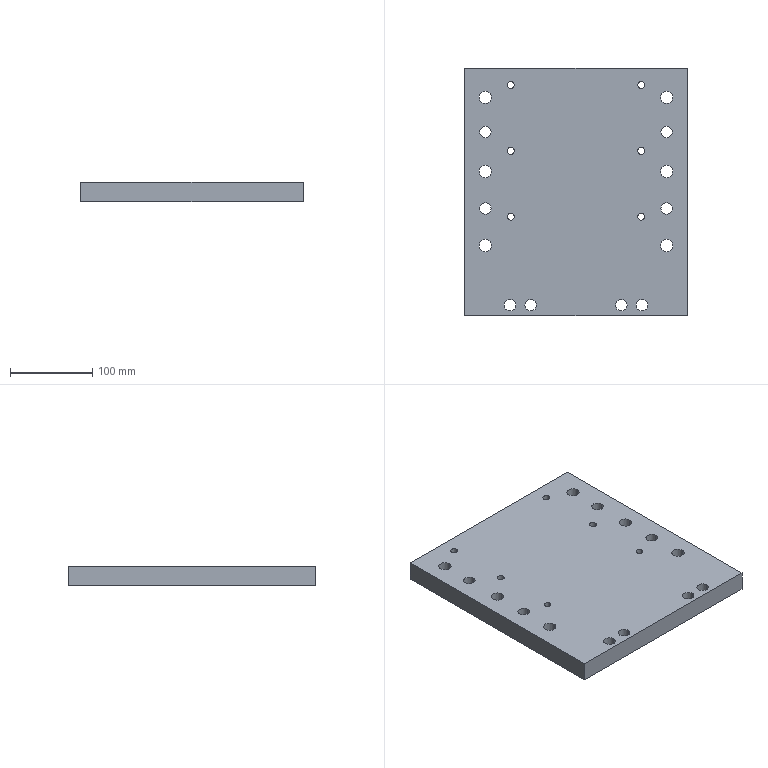Part | STEP file | TAM TRUOT DAU BUA GIUA | 1 solid | 46 faces | box 270 x 300 x 24 mm | volume 1881062 mm3 | cylinder 40 | plane 6 | commonest cylinder face diameters 14 x16 8.376 x12 15 x12